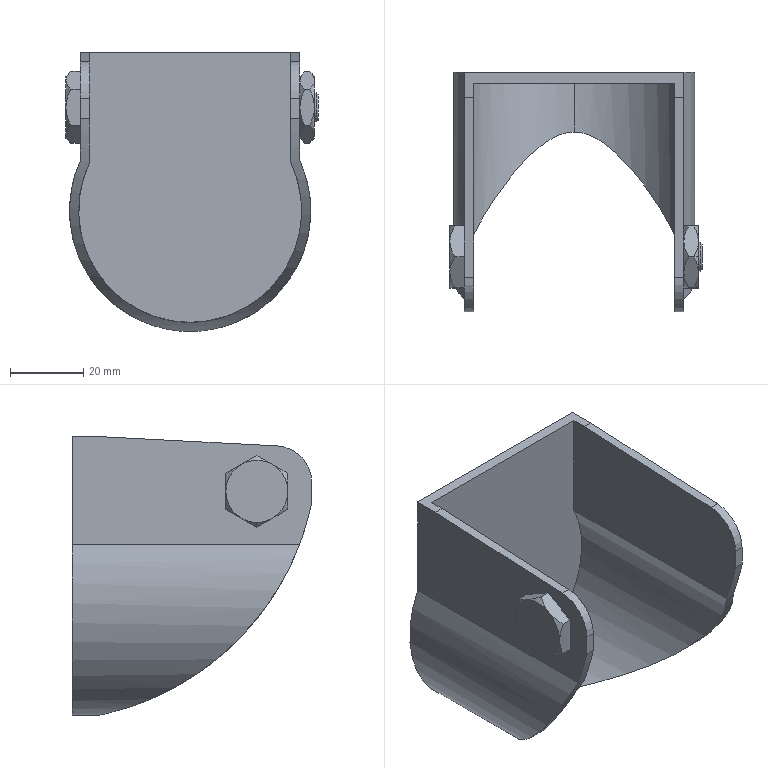Part | SolidWorks | features BaseBody 1 | 1 solid | 57 faces | box 69 x 65.5 x 76.3 mm | volume 35082 mm3 | plane 26 | cone 22 | cylinder 9 | commonest cylinder face diameters 8 x2 20 x2 61 x2 66 x2 150 x1